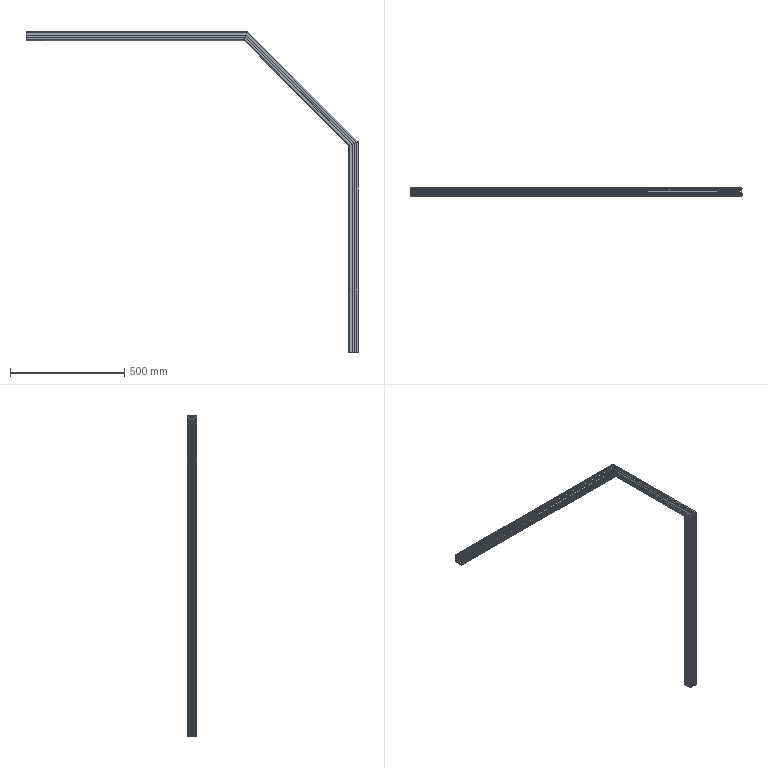Part | 3 solids | 312 faces | box 1450 x 40 x 1400 mm | volume 1461504 mm3 | plane 282 | cylinder 30 | commonest cylinder face diameters 5 x12 9 x12 6.8 x6